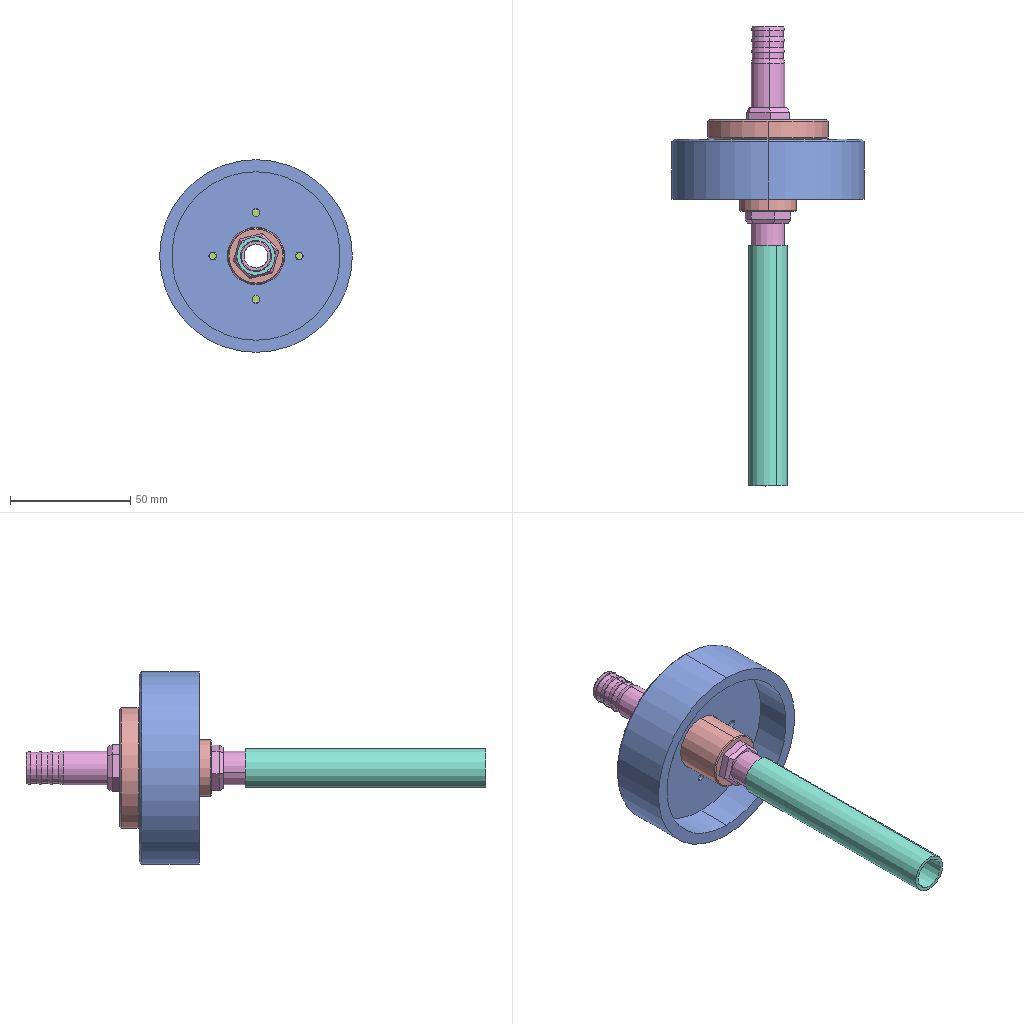Assembly | SolidWorks | 5 different items | 9 placed | box 80 x 191 x 80 mm
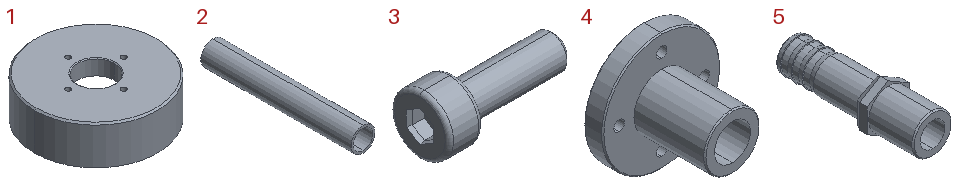Parts list (item | quantity | size | volume | features):
1 | x1 | 80 x 80 x 25 mm | 62937 mm3 | features Chamfer 2, 3DProfileFeature 1, HoleWzd 1, ICE 1, Revolution 1
2 | x1 | 16 x 100 x 16 mm | 6833 mm3 | features Sweep 1
3 | x4 | 16 x 7 x 7 mm | 285.121 mm3 | features Chamfer 2, Fillet 1, ICE 1, Revolution 1
4 | x1 | 50 x 38 x 50 mm | 20590 mm3 | features 3DProfileFeature 3, HoleWzd 3, Chamfer 1, Revolution 1
5 | x2 | 17 x 57 x 19.63 mm | 5326 mm3 | features ICE 3, Chamfer 2, Extrusion 1, Fillet 1, RevCut 1
Mates (type | each side: item.copy, entity, surface, feature):
Concentric | 4.1 face cylinder Revolve1 | 1.1 face cylinder Cut-Extrude1
Coincident | 4.1 face plane Revolve1 | 1.1 face plane Revolve2
Concentric | 4.1 face cylinder Hole Size (per socket head cap screw type)1 | 1.1 face cylinder M4 Tapped Hole1
Concentric | 4.1 face cylinder Hole Size (per socket head cap screw type)1 | 3.1 face cylinder Revolve1
Coincident | 4.1 face plane Hole Size (per socket head cap screw type)1 | 3.1 face plane Revolve1
Concentric | 4.1 face cylinder Hole Size (per socket head cap screw type)1 | 3.2 face cylinder Revolve1
Coincident | 4.1 face plane Hole Size (per socket head cap screw type)1 | 3.2 face plane Revolve1
Concentric | 4.1 face cylinder Hole Size (per socket head cap screw type)1 | 3.3 face cylinder Revolve1
Coincident | 4.1 face plane Hole Size (per socket head cap screw type)1 | 3.3 face plane Revolve1
Concentric | 4.1 face cylinder Hole Size (per socket head cap screw type)1 | 3.4 face cylinder Revolve1
Coincident | 4.1 face plane Hole Size (per socket head cap screw type)1 | 3.4 face plane Revolve1
Concentric | 4.1 face cylinder G3/8 Tapped Hole1 | 5.1 face cylinder Boss-Extrude3
Coincident | 4.1 face plane Revolve1 | 5.1 face plane Boss-Extrude2
Concentric | 5.1 face cylinder Boss-Extrude1 | 2.1 face cylinder Sweep-Thin Part1
Concentric | 4.1 face cylinder Revolve1 | 5.2 face cylinder Boss-Extrude3
Coincident | 4.1 face plane Revolve1 | 5.2 face plane Boss-Extrude2
DistanceDim | 2.1 face plane Sweep-Thin Part1 | 1.1 face plane Revolve2